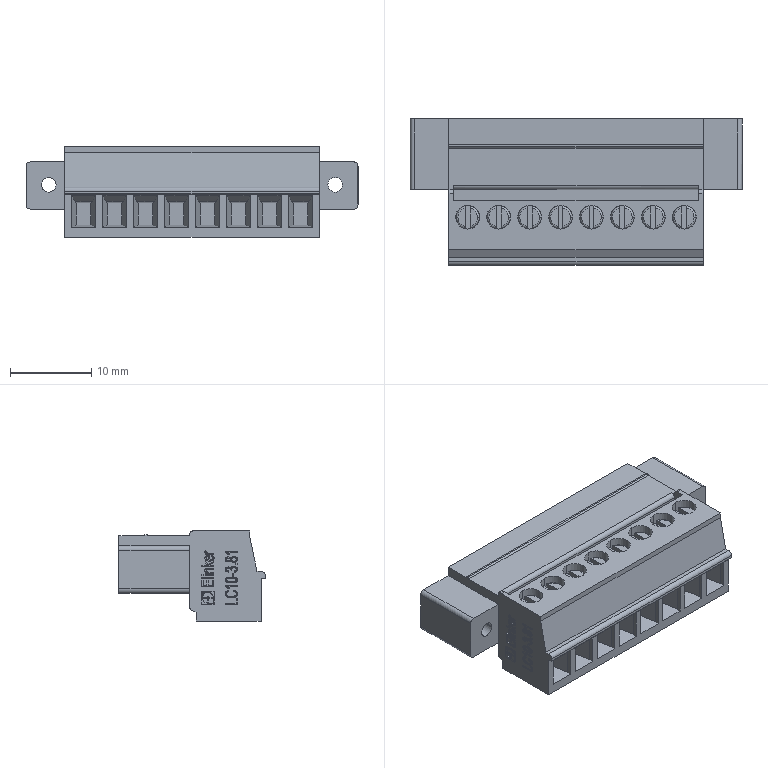Part | NX | features BREP 19 | 19 solids | 4092 faces | volume 4072 mm3 | plane 3741 | cylinder 181 | spline 94 | torus 64 | cone 12 | commonest cylinder face diameters 3.2 x40 3.6 x36 2 x16 2.8 x16 2.94 x16 2.2 x14